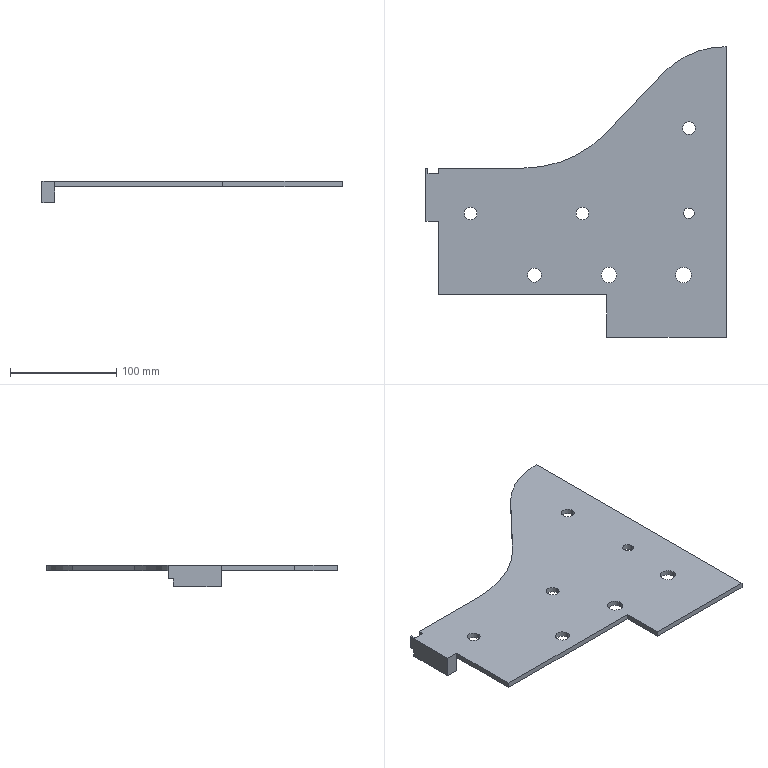Part | SolidWorks | features ICE 3, Cut 2, Extrusion 1 | 1 solid | 34 faces | box 282 x 273 x 20 mm | volume 241277 mm3 | plane 18 | cylinder 16 | commonest cylinder face diameters 12 x6 10 x2 13.206 x2 14.603 x2 14.666 x2 166 x1
STEP:
#1=CARTESIAN_POINT('',(55.96,-170.411,0.));
#2=VERTEX_POINT('',#1);
#3=CARTESIAN_POINT('',(70.625,-170.411,0.));
#4=VERTEX_POINT('',#3);
#5=CARTESIAN_POINT('',(63.293,-170.411,0.));
#6=DIRECTION('',(0.,0.,1.));
#7=DIRECTION('',(1.,0.,0.));
#8=AXIS2_PLACEMENT_3D('',#5,#6,#7);
#9=CIRCLE('',#8,7.333);
#10=EDGE_CURVE('',#2,#4,#9,.T.);
#11=ORIENTED_EDGE('',*,*,#10,.F.);
#12=CARTESIAN_POINT('',(55.96,-170.411,5.));
#13=VERTEX_POINT('',#12);
#14=CARTESIAN_POINT('',(55.96,-170.411,-50.741));
#15=DIRECTION('',(0.,0.,1.));
#16=VECTOR('',#15,1000.);
#17=LINE('',#14,#16);
#18=EDGE_CURVE('',#2,#13,#17,.T.);
#19=ORIENTED_EDGE('',*,*,#18,.T.);
#20=CARTESIAN_POINT('',(70.625,-170.411,5.));
#21=VERTEX_POINT('',#20);
#22=CARTESIAN_POINT('',(63.293,-170.411,5.));
#23=DIRECTION('',(0.,0.,1.));
#24=DIRECTION('',(1.,0.,0.));
#25=AXIS2_PLACEMENT_3D('',#22,#23,#24);
#26=CIRCLE('',#25,7.333);
#27=EDGE_CURVE('',#13,#21,#26,.T.);
#28=ORIENTED_EDGE('',*,*,#27,.T.);
#29=CARTESIAN_POINT('',(70.625,-170.411,-50.741));
#30=DIRECTION('',(0.,0.,1.));
#31=VECTOR('',#30,1000.);
#32=LINE('',#29,#31);
#33=EDGE_CURVE('',#4,#21,#32,.T.);
#34=ORIENTED_EDGE('',*,*,#33,.F.);
#35=EDGE_LOOP('',(#11,#19,#28,#34));
#36=FACE_OUTER_BOUND('',#35,.T.);
#37=CARTESIAN_POINT('',(63.293,-170.411,-50.741));
#38=DIRECTION('',(0.,0.,1.));
#39=DIRECTION('',(1.,0.,0.));
#40=AXIS2_PLACEMENT_3D('',#37,#38,#39);
#41=CYLINDRICAL_SURFACE('',#40,7.333);
#42=ADVANCED_FACE('',(#36),#41,.F.);
#43=CARTESIAN_POINT('',(-14.009,-170.411,0.));
#44=VERTEX_POINT('',#43);
#45=CARTESIAN_POINT('',(0.5938,-170.411,0.));
#46=VERTEX_POINT('',#45);
#47=CARTESIAN_POINT('',(-6.707,-170.411,0.));
#48=DIRECTION('',(0.,0.,1.));
#49=DIRECTION('',(1.,0.,0.));
#50=AXIS2_PLACEMENT_3D('',#47,#48,#49);
#51=CIRCLE('',#50,7.301);
#52=EDGE_CURVE('',#44,#46,#51,.T.);
#53=ORIENTED_EDGE('',*,*,#52,.F.);
#54=CARTESIAN_POINT('',(-14.009,-170.411,5.));
#55=VERTEX_POINT('',#54);
#56=CARTESIAN_POINT('',(-14.009,-170.411,-50.741));
#57=DIRECTION('',(0.,0.,1.));
#58=VECTOR('',#57,1000.);
#59=LINE('',#56,#58);
#60=EDGE_CURVE('',#44,#55,#59,.T.);
#61=ORIENTED_EDGE('',*,*,#60,.T.);
#62=CARTESIAN_POINT('',(0.5938,-170.411,5.));
#63=VERTEX_POINT('',#62);
#64=CARTESIAN_POINT('',(-6.707,-170.411,5.));
#65=DIRECTION('',(0.,0.,1.));
#66=DIRECTION('',(1.,0.,0.));
#67=AXIS2_PLACEMENT_3D('',#64,#65,#66);
#68=CIRCLE('',#67,7.301);
#69=EDGE_CURVE('',#55,#63,#68,.T.);
#70=ORIENTED_EDGE('',*,*,#69,.T.);
#71=CARTESIAN_POINT('',(0.5938,-170.411,-50.741));
#72=DIRECTION('',(0.,0.,1.));
#73=VECTOR('',#72,1000.);
#74=LINE('',#71,#73);
#75=EDGE_CURVE('',#46,#63,#74,.T.);
#76=ORIENTED_EDGE('',*,*,#75,.F.);
#77=EDGE_LOOP('',(#53,#61,#70,#76));
#78=FACE_OUTER_BOUND('',#77,.T.);
#79=CARTESIAN_POINT('',(-6.707,-170.411,-50.741));
#80=DIRECTION('',(0.,0.,1.));
#81=DIRECTION('',(1.,0.,0.));
#82=AXIS2_PLACEMENT_3D('',#79,#80,#81);
#83=CYLINDRICAL_SURFACE('',#82,7.301);
#84=ADVANCED_FACE('',(#78),#83,.F.);
#85=CARTESIAN_POINT('',(-83.311,-170.411,0.));
#86=VERTEX_POINT('',#85);
#87=CARTESIAN_POINT('',(-70.104,-170.411,0.));
#88=VERTEX_POINT('',#87);
#89=CARTESIAN_POINT('',(-76.707,-170.411,0.));
#90=DIRECTION('',(0.,0.,1.));
#91=DIRECTION('',(1.,0.,0.));
#92=AXIS2_PLACEMENT_3D('',#89,#90,#91);
#93=CIRCLE('',#92,6.603);
#94=EDGE_CURVE('',#86,#88,#93,.T.);
#95=ORIENTED_EDGE('',*,*,#94,.F.);
#96=CARTESIAN_POINT('',(-83.311,-170.411,5.));
#97=VERTEX_POINT('',#96);
#98=CARTESIAN_POINT('',(-83.311,-170.411,-50.741));
#99=DIRECTION('',(0.,0.,1.));
#100=VECTOR('',#99,1000.);
#101=LINE('',#98,#100);
#102=EDGE_CURVE('',#86,#97,#101,.T.);
#103=ORIENTED_EDGE('',*,*,#102,.T.);
#104=CARTESIAN_POINT('',(-70.104,-170.411,5.));
#105=VERTEX_POINT('',#104);
#106=CARTESIAN_POINT('',(-76.707,-170.411,5.));
#107=DIRECTION('',(0.,0.,1.));
#108=DIRECTION('',(1.,0.,0.));
#109=AXIS2_PLACEMENT_3D('',#106,#107,#108);
#110=CIRCLE('',#109,6.603);
#111=EDGE_CURVE('',#97,#105,#110,.T.);
#112=ORIENTED_EDGE('',*,*,#111,.T.);
#113=CARTESIAN_POINT('',(-70.104,-170.411,-50.741));
#114=DIRECTION('',(0.,0.,1.));
#115=VECTOR('',#114,1000.);
#116=LINE('',#113,#115);
#117=EDGE_CURVE('',#88,#105,#116,.T.);
#118=ORIENTED_EDGE('',*,*,#117,.F.);
#119=EDGE_LOOP('',(#95,#103,#112,#118));
#120=FACE_OUTER_BOUND('',#119,.T.);
#121=CARTESIAN_POINT('',(-76.707,-170.411,-50.741));
#122=DIRECTION('',(0.,0.,1.));
#123=DIRECTION('',(1.,0.,0.));
#124=AXIS2_PLACEMENT_3D('',#121,#122,#123);
#125=CYLINDRICAL_SURFACE('',#124,6.603);
#126=ADVANCED_FACE('',(#120),#125,.F.);
#127=CARTESIAN_POINT('',(62.293,-32.472,0.));
#128=VERTEX_POINT('',#127);
#129=CARTESIAN_POINT('',(74.293,-32.472,0.));
#130=VERTEX_POINT('',#129);
#131=CARTESIAN_POINT('',(68.293,-32.472,0.));
#132=DIRECTION('',(0.,0.,1.));
#133=DIRECTION('',(1.,0.,0.));
#134=AXIS2_PLACEMENT_3D('',#131,#132,#133);
#135=CIRCLE('',#134,6.);
#136=EDGE_CURVE('',#128,#130,#135,.T.);
#137=ORIENTED_EDGE('',*,*,#136,.F.);
#138=CARTESIAN_POINT('',(62.293,-32.472,5.));
#139=VERTEX_POINT('',#138);
#140=CARTESIAN_POINT('',(62.293,-32.472,-36.971));
#141=DIRECTION('',(0.,0.,1.));
#142=VECTOR('',#141,1000.);
#143=LINE('',#140,#142);
#144=EDGE_CURVE('',#128,#139,#143,.T.);
#145=ORIENTED_EDGE('',*,*,#144,.T.);
#146=CARTESIAN_POINT('',(74.293,-32.472,5.));
#147=VERTEX_POINT('',#146);
#148=CARTESIAN_POINT('',(68.293,-32.472,5.));
#149=DIRECTION('',(0.,0.,1.));
#150=DIRECTION('',(1.,0.,0.));
#151=AXIS2_PLACEMENT_3D('',#148,#149,#150);
#152=CIRCLE('',#151,6.);
#153=EDGE_CURVE('',#139,#147,#152,.T.);
#154=ORIENTED_EDGE('',*,*,#153,.T.);
#155=CARTESIAN_POINT('',(74.293,-32.472,-36.971));
#156=DIRECTION('',(0.,0.,1.));
#157=VECTOR('',#156,1000.);
#158=LINE('',#155,#157);
#159=EDGE_CURVE('',#130,#147,#158,.T.);
#160=ORIENTED_EDGE('',*,*,#159,.F.);
#161=EDGE_LOOP('',(#137,#145,#154,#160));
#162=FACE_OUTER_BOUND('',#161,.T.);
#163=CARTESIAN_POINT('',(68.293,-32.472,-36.971));
#164=DIRECTION('',(0.,0.,1.));
#165=DIRECTION('',(1.,0.,0.));
#166=AXIS2_PLACEMENT_3D('',#163,#164,#165);
#167=CYLINDRICAL_SURFACE('',#166,6.);
#168=ADVANCED_FACE('',(#162),#167,.F.);
#169=CARTESIAN_POINT('',(-142.707,-112.472,0.));
#170=VERTEX_POINT('',#169);
#171=CARTESIAN_POINT('',(-130.707,-112.472,0.));
#172=VERTEX_POINT('',#171);
#173=CARTESIAN_POINT('',(-136.707,-112.472,0.));
#174=DIRECTION('',(0.,0.,1.));
#175=DIRECTION('',(1.,0.,0.));
#176=AXIS2_PLACEMENT_3D('',#173,#174,#175);
#177=CIRCLE('',#176,6.);
#178=EDGE_CURVE('',#170,#172,#177,.T.);
#179=ORIENTED_EDGE('',*,*,#178,.F.);
#180=CARTESIAN_POINT('',(-142.707,-112.472,5.));
#181=VERTEX_POINT('',#180);
#182=CARTESIAN_POINT('',(-142.707,-112.472,-36.971));
#183=DIRECTION('',(0.,0.,1.));
#184=VECTOR('',#183,1000.);
#185=LINE('',#182,#184);
#186=EDGE_CURVE('',#170,#181,#185,.T.);
#187=ORIENTED_EDGE('',*,*,#186,.T.);
#188=CARTESIAN_POINT('',(-130.707,-112.472,5.));
#189=VERTEX_POINT('',#188);
#190=CARTESIAN_POINT('',(-136.707,-112.472,5.));
#191=DIRECTION('',(0.,0.,1.));
#192=DIRECTION('',(1.,0.,0.));
#193=AXIS2_PLACEMENT_3D('',#190,#191,#192);
#194=CIRCLE('',#193,6.);
#195=EDGE_CURVE('',#181,#189,#194,.T.);
#196=ORIENTED_EDGE('',*,*,#195,.T.);
#197=CARTESIAN_POINT('',(-130.707,-112.472,-36.971));
#198=DIRECTION('',(0.,0.,1.));
#199=VECTOR('',#198,1000.);
#200=LINE('',#197,#199);
#201=EDGE_CURVE('',#172,#189,#200,.T.);
#202=ORIENTED_EDGE('',*,*,#201,.F.);
#203=EDGE_LOOP('',(#179,#187,#196,#202));
#204=FACE_OUTER_BOUND('',#203,.T.);
#205=CARTESIAN_POINT('',(-136.707,-112.472,-36.971));
#206=DIRECTION('',(0.,0.,1.));
#207=DIRECTION('',(1.,0.,0.));
#208=AXIS2_PLACEMENT_3D('',#205,#206,#207);
#209=CYLINDRICAL_SURFACE('',#208,6.);
#210=ADVANCED_FACE('',(#204),#209,.F.);
#211=CARTESIAN_POINT('',(-37.707,-112.472,0.));
#212=VERTEX_POINT('',#211);
#213=CARTESIAN_POINT('',(-25.707,-112.472,0.));
#214=VERTEX_POINT('',#213);
#215=CARTESIAN_POINT('',(-31.707,-112.472,0.));
#216=DIRECTION('',(0.,0.,1.));
#217=DIRECTION('',(1.,0.,0.));
#218=AXIS2_PLACEMENT_3D('',#215,#216,#217);
#219=CIRCLE('',#218,6.);
#220=EDGE_CURVE('',#212,#214,#219,.T.);
#221=ORIENTED_EDGE('',*,*,#220,.F.);
#222=CARTESIAN_POINT('',(-37.707,-112.472,5.));
#223=VERTEX_POINT('',#222);
#224=CARTESIAN_POINT('',(-37.707,-112.472,-36.971));
#225=DIRECTION('',(0.,0.,1.));
#226=VECTOR('',#225,1000.);
#227=LINE('',#224,#226);
#228=EDGE_CURVE('',#212,#223,#227,.T.);
#229=ORIENTED_EDGE('',*,*,#228,.T.);
#230=CARTESIAN_POINT('',(-25.707,-112.472,5.));
#231=VERTEX_POINT('',#230);
#232=CARTESIAN_POINT('',(-31.707,-112.472,5.));
#233=DIRECTION('',(0.,0.,1.));
#234=DIRECTION('',(1.,0.,0.));
#235=AXIS2_PLACEMENT_3D('',#232,#233,#234);
#236=CIRCLE('',#235,6.);
#237=EDGE_CURVE('',#223,#231,#236,.T.);
#238=ORIENTED_EDGE('',*,*,#237,.T.);
#239=CARTESIAN_POINT('',(-25.707,-112.472,-36.971));
#240=DIRECTION('',(0.,0.,1.));
#241=VECTOR('',#240,1000.);
#242=LINE('',#239,#241);
#243=EDGE_CURVE('',#214,#231,#242,.T.);
#244=ORIENTED_EDGE('',*,*,#243,.F.);
#245=EDGE_LOOP('',(#221,#229,#238,#244));
#246=FACE_OUTER_BOUND('',#245,.T.);
#247=CARTESIAN_POINT('',(-31.707,-112.472,-36.971));
#248=DIRECTION('',(0.,0.,1.));
#249=DIRECTION('',(1.,0.,0.));
#250=AXIS2_PLACEMENT_3D('',#247,#248,#249);
#251=CYLINDRICAL_SURFACE('',#250,6.);
#252=ADVANCED_FACE('',(#246),#251,.F.);
#253=CARTESIAN_POINT('',(63.293,-112.472,0.));
#254=VERTEX_POINT('',#253);
#255=CARTESIAN_POINT('',(73.293,-112.472,0.));
#256=VERTEX_POINT('',#255);
#257=CARTESIAN_POINT('',(68.293,-112.472,0.));
#258=DIRECTION('',(0.,0.,1.));
#259=DIRECTION('',(1.,0.,0.));
#260=AXIS2_PLACEMENT_3D('',#257,#258,#259);
#261=CIRCLE('',#260,5.);
#262=EDGE_CURVE('',#254,#256,#261,.T.);
#263=ORIENTED_EDGE('',*,*,#262,.F.);
#264=CARTESIAN_POINT('',(63.293,-112.472,5.));
#265=VERTEX_POINT('',#264);
#266=CARTESIAN_POINT('',(63.293,-112.472,-36.971));
#267=DIRECTION('',(0.,0.,1.));
#268=VECTOR('',#267,1000.);
#269=LINE('',#266,#268);
#270=EDGE_CURVE('',#254,#265,#269,.T.);
#271=ORIENTED_EDGE('',*,*,#270,.T.);
#272=CARTESIAN_POINT('',(73.293,-112.472,5.));
#273=VERTEX_POINT('',#272);
#274=CARTESIAN_POINT('',(68.293,-112.472,5.));
#275=DIRECTION('',(0.,0.,1.));
#276=DIRECTION('',(1.,0.,0.));
#277=AXIS2_PLACEMENT_3D('',#274,#275,#276);
#278=CIRCLE('',#277,5.);
#279=EDGE_CURVE('',#265,#273,#278,.T.);
#280=ORIENTED_EDGE('',*,*,#279,.T.);
#281=CARTESIAN_POINT('',(73.293,-112.472,-36.971));
#282=DIRECTION('',(0.,0.,1.));
#283=VECTOR('',#282,1000.);
#284=LINE('',#281,#283);
#285=EDGE_CURVE('',#256,#273,#284,.T.);
#286=ORIENTED_EDGE('',*,*,#285,.F.);
#287=EDGE_LOOP('',(#263,#271,#280,#286));
#288=FACE_OUTER_BOUND('',#287,.T.);
#289=CARTESIAN_POINT('',(68.293,-112.472,-36.971));
#290=DIRECTION('',(0.,0.,1.));
#291=DIRECTION('',(1.,0.,0.));
#292=AXIS2_PLACEMENT_3D('',#289,#290,#291);
#293=CYLINDRICAL_SURFACE('',#292,5.);
#294=ADVANCED_FACE('',(#288),#293,.F.);
#295=CARTESIAN_POINT('',(-8.707,-188.911,5.));
#296=VERTEX_POINT('',#295);
#297=CARTESIAN_POINT('',(-8.707,-188.911,0.));
#298=VERTEX_POINT('',#297);
#299=CARTESIAN_POINT('',(-8.707,-188.911,5.));
#300=DIRECTION('',(0.,0.,-1.));
#301=VECTOR('',#300,1000.);
#302=LINE('',#299,#301);
#303=EDGE_CURVE('',#296,#298,#302,.T.);
#304=ORIENTED_EDGE('',*,*,#303,.F.);
#305=CARTESIAN_POINT('',(-166.707,-188.911,5.));
#306=VERTEX_POINT('',#305);
#307=CARTESIAN_POINT('',(-166.707,-188.911,5.));
#308=DIRECTION('',(1.,0.,0.));
#309=VECTOR('',#308,1000.);
#310=LINE('',#307,#309);
#311=EDGE_CURVE('',#306,#296,#310,.T.);
#312=ORIENTED_EDGE('',*,*,#311,.F.);
#313=CARTESIAN_POINT('',(-166.707,-188.911,0.));
#314=VERTEX_POINT('',#313);
#315=CARTESIAN_POINT('',(-166.707,-188.911,5.));
#316=DIRECTION('',(0.,0.,-1.));
#317=VECTOR('',#316,1000.);
#318=LINE('',#315,#317);
#319=EDGE_CURVE('',#306,#314,#318,.T.);
#320=ORIENTED_EDGE('',*,*,#319,.T.);
#321=CARTESIAN_POINT('',(-86.707,-188.911,0.));
#322=DIRECTION('',(1.,0.,0.));
#323=VECTOR('',#322,1000.);
#324=LINE('',#321,#323);
#325=EDGE_CURVE('',#314,#298,#324,.T.);
#326=ORIENTED_EDGE('',*,*,#325,.T.);
#327=EDGE_LOOP('',(#304,#312,#320,#326));
#328=FACE_OUTER_BOUND('',#327,.T.);
#329=CARTESIAN_POINT('',(-86.707,-188.911,5.));
#330=DIRECTION('',(0.,1.,0.));
#331=DIRECTION('',(0.,0.,1.));
#332=AXIS2_PLACEMENT_3D('',#329,#330,#331);
#333=PLANE('',#332);
#334=ADVANCED_FACE('',(#328),#333,.F.);
#335=CARTESIAN_POINT('',(-166.707,-69.911,5.));
#336=VERTEX_POINT('',#335);
#337=CARTESIAN_POINT('',(-166.707,-69.911,0.));
#338=VERTEX_POINT('',#337);
#339=CARTESIAN_POINT('',(-166.707,-69.911,0.));
#340=DIRECTION('',(0.,0.,-1.));
#341=VECTOR('',#340,1000.);
#342=LINE('',#339,#341);
#343=EDGE_CURVE('',#336,#338,#342,.T.);
#344=ORIENTED_EDGE('',*,*,#343,.F.);
#345=CARTESIAN_POINT('',(-86.707,-69.911,5.));
#346=VERTEX_POINT('',#345);
#347=CARTESIAN_POINT('',(-166.707,-69.911,5.));
#348=DIRECTION('',(1.,0.,0.));
#349=VECTOR('',#348,1000.);
#350=LINE('',#347,#349);
#351=EDGE_CURVE('',#336,#346,#350,.T.);
#352=ORIENTED_EDGE('',*,*,#351,.T.);
#353=CARTESIAN_POINT('',(-86.707,-69.911,0.));
#354=VERTEX_POINT('',#353);
#355=CARTESIAN_POINT('',(-86.707,-69.911,5.));
#356=DIRECTION('',(0.,0.,-1.));
#357=VECTOR('',#356,1000.);
#358=LINE('',#355,#357);
#359=EDGE_CURVE('',#346,#354,#358,.T.);
#360=ORIENTED_EDGE('',*,*,#359,.T.);
#361=CARTESIAN_POINT('',(-166.707,-69.911,0.));
#362=DIRECTION('',(1.,0.,0.));
#363=VECTOR('',#362,1000.);
#364=LINE('',#361,#363);
#365=EDGE_CURVE('',#338,#354,#364,.T.);
#366=ORIENTED_EDGE('',*,*,#365,.F.);
#367=EDGE_LOOP('',(#344,#352,#360,#366));
#368=FACE_OUTER_BOUND('',#367,.T.);
#369=CARTESIAN_POINT('',(-166.707,-69.911,5.));
#370=DIRECTION('',(0.,1.,0.));
#371=DIRECTION('',(0.,0.,1.));
#372=AXIS2_PLACEMENT_3D('',#369,#370,#371);
#373=PLANE('',#372);
#374=ADVANCED_FACE('',(#368),#373,.T.);
#375=CARTESIAN_POINT('',(-166.707,-119.911,5.));
#376=VERTEX_POINT('',#375);
#377=CARTESIAN_POINT('',(-166.707,-69.911,5.));
#378=DIRECTION('',(0.,-1.,0.));
#379=VECTOR('',#378,1000.);
#380=LINE('',#377,#379);
#381=EDGE_CURVE('',#376,#306,#380,.T.);
#382=ORIENTED_EDGE('',*,*,#381,.F.);
#383=CARTESIAN_POINT('',(-166.707,-119.911,0.));
#384=VERTEX_POINT('',#383);
#385=CARTESIAN_POINT('',(-166.707,-119.911,5.));
#386=DIRECTION('',(0.,0.,-1.));
#387=VECTOR('',#386,1000.);
#388=LINE('',#385,#387);
#389=EDGE_CURVE('',#376,#384,#388,.T.);
#390=ORIENTED_EDGE('',*,*,#389,.T.);
#391=CARTESIAN_POINT('',(-166.707,-69.911,0.));
#392=DIRECTION('',(0.,-1.,0.));
#393=VECTOR('',#392,1000.);
#394=LINE('',#391,#393);
#395=EDGE_CURVE('',#384,#314,#394,.T.);
#396=ORIENTED_EDGE('',*,*,#395,.T.);
#397=ORIENTED_EDGE('',*,*,#319,.F.);
#398=EDGE_LOOP('',(#382,#390,#396,#397));
#399=FACE_OUTER_BOUND('',#398,.T.);
#400=CARTESIAN_POINT('',(-166.707,-69.911,5.));
#401=DIRECTION('',(1.,0.,0.));
#402=DIRECTION('',(0.,0.,-1.));
#403=AXIS2_PLACEMENT_3D('',#400,#401,#402);
#404=PLANE('',#403);
#405=ADVANCED_FACE('',(#399),#404,.F.);
#406=CARTESIAN_POINT('',(103.293,44.089,0.));
#407=VERTEX_POINT('',#406);
#408=CARTESIAN_POINT('',(103.293,-228.911,0.));
#409=VERTEX_POINT('',#408);
#410=CARTESIAN_POINT('',(103.293,44.089,0.));
#411=DIRECTION('',(0.,-1.,0.));
#412=VECTOR('',#411,1000.);
#413=LINE('',#410,#412);
#414=EDGE_CURVE('',#407,#409,#413,.T.);
#415=ORIENTED_EDGE('',*,*,#414,.F.);
#416=CARTESIAN_POINT('',(103.293,44.089,5.));
#417=VERTEX_POINT('',#416);
#418=CARTESIAN_POINT('',(103.293,44.089,5.));
#419=DIRECTION('',(0.,0.,-1.));
#420=VECTOR('',#419,1000.);
#421=LINE('',#418,#420);
#422=EDGE_CURVE('',#417,#407,#421,.T.);
#423=ORIENTED_EDGE('',*,*,#422,.F.);
#424=CARTESIAN_POINT('',(103.293,-228.911,5.));
#425=VERTEX_POINT('',#424);
#426=CARTESIAN_POINT('',(103.293,44.089,5.));
#427=DIRECTION('',(0.,-1.,0.));
#428=VECTOR('',#427,1000.);
#429=LINE('',#426,#428);
#430=EDGE_CURVE('',#417,#425,#429,.T.);
#431=ORIENTED_EDGE('',*,*,#430,.T.);
#432=CARTESIAN_POINT('',(103.293,-228.911,5.));
#433=DIRECTION('',(0.,0.,1.));
#434=VECTOR('',#433,1000.);
#435=LINE('',#432,#434);
#436=EDGE_CURVE('',#409,#425,#435,.T.);
#437=ORIENTED_EDGE('',*,*,#436,.F.);
#438=EDGE_LOOP('',(#415,#423,#431,#437));
#439=FACE_OUTER_BOUND('',#438,.T.);
#440=CARTESIAN_POINT('',(103.293,44.089,5.));
#441=DIRECTION('',(1.,0.,0.));
#442=DIRECTION('',(0.,0.,-1.));
#443=AXIS2_PLACEMENT_3D('',#440,#441,#442);
#444=PLANE('',#443);
#445=ADVANCED_FACE('',(#439),#444,.T.);
#446=CARTESIAN_POINT('',(44.7,19.876,0.));
#447=VERTEX_POINT('',#446);
#448=CARTESIAN_POINT('',(103.293,-38.911,0.));
#449=DIRECTION('',(0.,0.,1.));
#450=DIRECTION('',(1.,0.,0.));
#451=AXIS2_PLACEMENT_3D('',#448,#449,#450);
#452=CIRCLE('',#451,83.);
#453=EDGE_CURVE('',#407,#447,#452,.T.);
#454=ORIENTED_EDGE('',*,*,#453,.T.);
#455=CARTESIAN_POINT('',(44.7,19.876,5.));
#456=VERTEX_POINT('',#455);
#457=CARTESIAN_POINT('',(44.7,19.876,5.));
#458=DIRECTION('',(0.,0.,-1.));
#459=VECTOR('',#458,1000.);
#460=LINE('',#457,#459);
#461=EDGE_CURVE('',#456,#447,#460,.T.);
#462=ORIENTED_EDGE('',*,*,#461,.F.);
#463=CARTESIAN_POINT('',(103.293,-38.911,5.));
#464=DIRECTION('',(0.,0.,1.));
#465=DIRECTION('',(1.,0.,0.));
#466=AXIS2_PLACEMENT_3D('',#463,#464,#465);
#467=CIRCLE('',#466,83.);
#468=EDGE_CURVE('',#417,#456,#467,.T.);
#469=ORIENTED_EDGE('',*,*,#468,.F.);
#470=ORIENTED_EDGE('',*,*,#422,.T.);
#471=EDGE_LOOP('',(#454,#462,#469,#470));
#472=FACE_OUTER_BOUND('',#471,.T.);
#473=CARTESIAN_POINT('',(103.293,-38.911,5.));
#474=DIRECTION('',(0.,0.,-1.));
#475=DIRECTION('',(-1.,0.,0.));
#476=AXIS2_PLACEMENT_3D('',#473,#474,#475);
#477=CYLINDRICAL_SURFACE('',#476,83.);
#478=ADVANCED_FACE('',(#472),#477,.T.);
#479=CARTESIAN_POINT('',(-10.944,-38.467,0.));
#480=VERTEX_POINT('',#479);
#481=CARTESIAN_POINT('',(-10.944,-38.467,0.));
#482=CARTESIAN_POINT('',(16.878,-9.296,0.));
#483=CARTESIAN_POINT('',(44.7,19.876,0.));
#484=B_SPLINE_CURVE_WITH_KNOTS('',2,(#481,#482,#483),.UNSPECIFIED.,.F.,.F.,(3,3),(-0.00171,0.9982),.UNSPECIFIED.);
#485=EDGE_CURVE('',#480,#447,#484,.T.);
#486=ORIENTED_EDGE('',*,*,#485,.F.);
#487=CARTESIAN_POINT('',(-10.944,-38.467,5.));
#488=VERTEX_POINT('',#487);
#489=CARTESIAN_POINT('',(-10.944,-38.467,5.));
#490=DIRECTION('',(0.,0.,-1.));
#491=VECTOR('',#490,1000.);
#492=LINE('',#489,#491);
#493=EDGE_CURVE('',#488,#480,#492,.T.);
#494=ORIENTED_EDGE('',*,*,#493,.F.);
#495=CARTESIAN_POINT('',(-10.944,-38.467,5.));
#496=CARTESIAN_POINT('',(16.878,-9.296,5.));
#497=CARTESIAN_POINT('',(44.7,19.876,5.));
#498=B_SPLINE_CURVE_WITH_KNOTS('',2,(#495,#496,#497),.UNSPECIFIED.,.F.,.F.,(3,3),(-0.00171,0.9982),.UNSPECIFIED.);
#499=EDGE_CURVE('',#488,#456,#498,.T.);
#500=ORIENTED_EDGE('',*,*,#499,.T.);
#501=ORIENTED_EDGE('',*,*,#461,.T.);
#502=EDGE_LOOP('',(#486,#494,#500,#501));
#503=FACE_OUTER_BOUND('',#502,.T.);
#504=CARTESIAN_POINT('',(-10.944,-38.467,5.));
#505=DIRECTION('',(-0.7237,0.6902,0.));
#506=DIRECTION('',(-0.6902,-0.7237,0.));
#507=AXIS2_PLACEMENT_3D('',#504,#505,#506);
#508=PLANE('',#507);
#509=ADVANCED_FACE('',(#503),#508,.T.);
#510=CARTESIAN_POINT('',(-86.707,37.089,0.));
#511=DIRECTION('',(0.,0.,1.));
#512=DIRECTION('',(1.,0.,0.));
#513=AXIS2_PLACEMENT_3D('',#510,#511,#512);
#514=CIRCLE('',#513,107.);
#515=EDGE_CURVE('',#354,#480,#514,.T.);
#516=ORIENTED_EDGE('',*,*,#515,.F.);
#517=ORIENTED_EDGE('',*,*,#359,.F.);
#518=CARTESIAN_POINT('',(-86.707,37.089,5.));
#519=DIRECTION('',(0.,0.,1.));
#520=DIRECTION('',(1.,0.,0.));
#521=AXIS2_PLACEMENT_3D('',#518,#519,#520);
#522=CIRCLE('',#521,107.);
#523=EDGE_CURVE('',#346,#488,#522,.T.);
#524=ORIENTED_EDGE('',*,*,#523,.T.);
#525=ORIENTED_EDGE('',*,*,#493,.T.);
#526=EDGE_LOOP('',(#516,#517,#524,#525));
#527=FACE_OUTER_BOUND('',#526,.T.);
#528=CARTESIAN_POINT('',(-86.707,37.089,5.));
#529=DIRECTION('',(0.,0.,-1.));
#530=DIRECTION('',(-1.,0.,0.));
#531=AXIS2_PLACEMENT_3D('',#528,#529,#530);
#532=CYLINDRICAL_SURFACE('',#531,107.);
#533=ADVANCED_FACE('',(#527),#532,.F.);
#534=CARTESIAN_POINT('',(-176.72,-69.911,-7.5));
#535=VERTEX_POINT('',#534);
#536=CARTESIAN_POINT('',(-176.72,-69.911,5.));
#537=VERTEX_POINT('',#536);
#538=CARTESIAN_POINT('',(-176.72,-69.911,5.));
#539=DIRECTION('',(0.,0.,1.));
#540=VECTOR('',#539,1000.);
#541=LINE('',#538,#540);
#542=EDGE_CURVE('',#535,#537,#541,.T.);
#543=ORIENTED_EDGE('',*,*,#542,.F.);
#544=CARTESIAN_POINT('',(-178.707,-69.911,-7.5));
#545=VERTEX_POINT('',#544);
#546=CARTESIAN_POINT('',(-176.72,-69.911,-7.5));
#547=DIRECTION('',(1.,0.,0.));
#548=VECTOR('',#547,1000.);
#549=LINE('',#546,#548);
#550=EDGE_CURVE('',#545,#535,#549,.T.);
#551=ORIENTED_EDGE('',*,*,#550,.F.);
#552=CARTESIAN_POINT('',(-178.707,-69.911,5.));
#553=VERTEX_POINT('',#552);
#554=CARTESIAN_POINT('',(-178.707,-69.911,5.));
#555=DIRECTION('',(0.,0.,1.));
#556=VECTOR('',#555,1000.);
#557=LINE('',#554,#556);
#558=EDGE_CURVE('',#545,#553,#557,.T.);
#559=ORIENTED_EDGE('',*,*,#558,.T.);
#560=CARTESIAN_POINT('',(-166.707,-69.911,5.));
#561=DIRECTION('',(1.,0.,0.));
#562=VECTOR('',#561,1000.);
#563=LINE('',#560,#562);
#564=EDGE_CURVE('',#553,#537,#563,.T.);
#565=ORIENTED_EDGE('',*,*,#564,.T.);
#566=EDGE_LOOP('',(#543,#551,#559,#565));
#567=FACE_OUTER_BOUND('',#566,.T.);
#568=CARTESIAN_POINT('',(-166.707,-69.911,5.));
#569=DIRECTION('',(0.,1.,0.));
#570=DIRECTION('',(0.,0.,1.));
#571=AXIS2_PLACEMENT_3D('',#568,#569,#570);
#572=PLANE('',#571);
#573=ADVANCED_FACE('',(#567),#572,.T.);
#574=CARTESIAN_POINT('',(63.293,-170.411,5.));
#575=DIRECTION('',(0.,0.,1.));
#576=DIRECTION('',(1.,0.,0.));
#577=AXIS2_PLACEMENT_3D('',#574,#575,#576);
#578=CIRCLE('',#577,7.333);
#579=EDGE_CURVE('',#21,#13,#578,.T.);
#580=ORIENTED_EDGE('',*,*,#579,.F.);
#581=ORIENTED_EDGE('',*,*,#27,.F.);
#582=EDGE_LOOP('',(#580,#581));
#583=FACE_BOUND('',#582,.T.);
#584=CARTESIAN_POINT('',(-6.707,-170.411,5.));
#585=DIRECTION('',(0.,0.,1.));
#586=DIRECTION('',(1.,0.,0.));
#587=AXIS2_PLACEMENT_3D('',#584,#585,#586);
#588=CIRCLE('',#587,7.301);
#589=EDGE_CURVE('',#63,#55,#588,.T.);
#590=ORIENTED_EDGE('',*,*,#589,.F.);
#591=ORIENTED_EDGE('',*,*,#69,.F.);
#592=EDGE_LOOP('',(#590,#591));
#593=FACE_BOUND('',#592,.T.);
#594=CARTESIAN_POINT('',(-76.707,-170.411,5.));
#595=DIRECTION('',(0.,0.,1.));
#596=DIRECTION('',(1.,0.,0.));
#597=AXIS2_PLACEMENT_3D('',#594,#595,#596);
#598=CIRCLE('',#597,6.603);
#599=EDGE_CURVE('',#105,#97,#598,.T.);
#600=ORIENTED_EDGE('',*,*,#599,.F.);
#601=ORIENTED_EDGE('',*,*,#111,.F.);
#602=EDGE_LOOP('',(#600,#601));
#603=FACE_BOUND('',#602,.T.);
#604=CARTESIAN_POINT('',(68.293,-32.472,5.));
#605=DIRECTION('',(0.,0.,1.));
#606=DIRECTION('',(1.,0.,0.));
#607=AXIS2_PLACEMENT_3D('',#604,#605,#606);
#608=CIRCLE('',#607,6.);
#609=EDGE_CURVE('',#147,#139,#608,.T.);
#610=ORIENTED_EDGE('',*,*,#609,.F.);
#611=ORIENTED_EDGE('',*,*,#153,.F.);
#612=EDGE_LOOP('',(#610,#611));
#613=FACE_BOUND('',#612,.T.);
#614=CARTESIAN_POINT('',(-136.707,-112.472,5.));
#615=DIRECTION('',(0.,0.,1.));
#616=DIRECTION('',(1.,0.,0.));
#617=AXIS2_PLACEMENT_3D('',#614,#615,#616);
#618=CIRCLE('',#617,6.);
#619=EDGE_CURVE('',#189,#181,#618,.T.);
#620=ORIENTED_EDGE('',*,*,#619,.F.);
#621=ORIENTED_EDGE('',*,*,#195,.F.);
#622=EDGE_LOOP('',(#620,#621));
#623=FACE_BOUND('',#622,.T.);
#624=CARTESIAN_POINT('',(-31.707,-112.472,5.));
#625=DIRECTION('',(0.,0.,1.));
#626=DIRECTION('',(1.,0.,0.));
#627=AXIS2_PLACEMENT_3D('',#624,#625,#626);
#628=CIRCLE('',#627,6.);
#629=EDGE_CURVE('',#231,#223,#628,.T.);
#630=ORIENTED_EDGE('',*,*,#629,.F.);
#631=ORIENTED_EDGE('',*,*,#237,.F.);
#632=EDGE_LOOP('',(#630,#631));
#633=FACE_BOUND('',#632,.T.);
#634=CARTESIAN_POINT('',(68.293,-112.472,5.));
#635=DIRECTION('',(0.,0.,1.));
#636=DIRECTION('',(1.,0.,0.));
#637=AXIS2_PLACEMENT_3D('',#634,#635,#636);
#638=CIRCLE('',#637,5.);
#639=EDGE_CURVE('',#273,#265,#638,.T.);
#640=ORIENTED_EDGE('',*,*,#639,.F.);
#641=ORIENTED_EDGE('',*,*,#279,.F.);
#642=EDGE_LOOP('',(#640,#641));
#643=FACE_BOUND('',#642,.T.);
#644=CARTESIAN_POINT('',(-166.707,-74.911,5.));
#645=VERTEX_POINT('',#644);
#646=CARTESIAN_POINT('',(-166.707,-74.911,5.));
#647=DIRECTION('',(0.,1.,0.));
#648=VECTOR('',#647,1000.);
#649=LINE('',#646,#648);
#650=EDGE_CURVE('',#645,#336,#649,.T.);
#651=ORIENTED_EDGE('',*,*,#650,.F.);
#652=CARTESIAN_POINT('',(-176.72,-74.911,5.));
#653=VERTEX_POINT('',#652);
#654=CARTESIAN_POINT('',(-166.707,-74.911,5.));
#655=DIRECTION('',(1.,0.,0.));
#656=VECTOR('',#655,1000.);
#657=LINE('',#654,#656);
#658=EDGE_CURVE('',#653,#645,#657,.T.);
#659=ORIENTED_EDGE('',*,*,#658,.F.);
#660=CARTESIAN_POINT('',(-176.72,-74.911,5.));
#661=DIRECTION('',(0.,1.,0.));
#662=VECTOR('',#661,1000.);
#663=LINE('',#660,#662);
#664=EDGE_CURVE('',#653,#537,#663,.T.);
#665=ORIENTED_EDGE('',*,*,#664,.T.);
#666=ORIENTED_EDGE('',*,*,#564,.F.);
#667=CARTESIAN_POINT('',(-178.707,-119.911,5.));
#668=VERTEX_POINT('',#667);
#669=CARTESIAN_POINT('',(-178.707,-119.911,5.));
#670=DIRECTION('',(0.,1.,0.));
#671=VECTOR('',#670,1000.);
#672=LINE('',#669,#671);
#673=EDGE_CURVE('',#668,#553,#672,.T.);
#674=ORIENTED_EDGE('',*,*,#673,.F.);
#675=CARTESIAN_POINT('',(-166.707,-119.911,5.));
#676=DIRECTION('',(1.,0.,0.));
#677=VECTOR('',#676,1000.);
#678=LINE('',#675,#677);
#679=EDGE_CURVE('',#668,#376,#678,.T.);
#680=ORIENTED_EDGE('',*,*,#679,.T.);
#681=ORIENTED_EDGE('',*,*,#381,.T.);
#682=ORIENTED_EDGE('',*,*,#311,.T.);
#683=CARTESIAN_POINT('',(-8.707,-228.911,5.));
#684=VERTEX_POINT('',#683);
#685=CARTESIAN_POINT('',(-8.707,-228.911,5.));
#686=DIRECTION('',(0.,1.,0.));
#687=VECTOR('',#686,1000.);
#688=LINE('',#685,#687);
#689=EDGE_CURVE('',#684,#296,#688,.T.);
#690=ORIENTED_EDGE('',*,*,#689,.F.);
#691=CARTESIAN_POINT('',(103.293,-228.911,5.));
#692=DIRECTION('',(-1.,0.,0.));
#693=VECTOR('',#692,1000.);
#694=LINE('',#691,#693);
#695=EDGE_CURVE('',#425,#684,#694,.T.);
#696=ORIENTED_EDGE('',*,*,#695,.F.);
#697=ORIENTED_EDGE('',*,*,#430,.F.);
#698=ORIENTED_EDGE('',*,*,#468,.T.);
#699=ORIENTED_EDGE('',*,*,#499,.F.);
#700=ORIENTED_EDGE('',*,*,#523,.F.);
#701=ORIENTED_EDGE('',*,*,#351,.F.);
#702=EDGE_LOOP('',(#651,#659,#665,#666,#674,#680,#681,#682,#690,#696,#697,#698,#699,#700,#701));
#703=FACE_OUTER_BOUND('',#702,.T.);
#704=CARTESIAN_POINT('',(103.293,-38.911,5.));
#705=DIRECTION('',(0.,0.,1.));
#706=DIRECTION('',(1.,0.,0.));
#707=AXIS2_PLACEMENT_3D('',#704,#705,#706);
#708=PLANE('',#707);
#709=ADVANCED_FACE('',(#583,#593,#603,#613,#623,#633,#643,#703),#708,.T.);
#710=CARTESIAN_POINT('',(63.293,-170.411,0.));
#711=DIRECTION('',(0.,0.,1.));
#712=DIRECTION('',(1.,0.,0.));
#713=AXIS2_PLACEMENT_3D('',#710,#711,#712);
#714=CIRCLE('',#713,7.333);
#715=EDGE_CURVE('',#4,#2,#714,.T.);
#716=ORIENTED_EDGE('',*,*,#715,.T.);
#717=ORIENTED_EDGE('',*,*,#10,.T.);
#718=EDGE_LOOP('',(#716,#717));
#719=FACE_BOUND('',#718,.T.);
#720=CARTESIAN_POINT('',(-6.707,-170.411,0.));
#721=DIRECTION('',(0.,0.,1.));
#722=DIRECTION('',(1.,0.,0.));
#723=AXIS2_PLACEMENT_3D('',#720,#721,#722);
#724=CIRCLE('',#723,7.301);
#725=EDGE_CURVE('',#46,#44,#724,.T.);
#726=ORIENTED_EDGE('',*,*,#725,.T.);
#727=ORIENTED_EDGE('',*,*,#52,.T.);
#728=EDGE_LOOP('',(#726,#727));
#729=FACE_BOUND('',#728,.T.);
#730=CARTESIAN_POINT('',(-76.707,-170.411,0.));
#731=DIRECTION('',(0.,0.,1.));
#732=DIRECTION('',(1.,0.,0.));
#733=AXIS2_PLACEMENT_3D('',#730,#731,#732);
#734=CIRCLE('',#733,6.603);
#735=EDGE_CURVE('',#88,#86,#734,.T.);
#736=ORIENTED_EDGE('',*,*,#735,.T.);
#737=ORIENTED_EDGE('',*,*,#94,.T.);
#738=EDGE_LOOP('',(#736,#737));
#739=FACE_BOUND('',#738,.T.);
#740=CARTESIAN_POINT('',(68.293,-32.472,0.));
#741=DIRECTION('',(0.,0.,1.));
#742=DIRECTION('',(1.,0.,0.));
#743=AXIS2_PLACEMENT_3D('',#740,#741,#742);
#744=CIRCLE('',#743,6.);
#745=EDGE_CURVE('',#130,#128,#744,.T.);
#746=ORIENTED_EDGE('',*,*,#745,.T.);
#747=ORIENTED_EDGE('',*,*,#136,.T.);
#748=EDGE_LOOP('',(#746,#747));
#749=FACE_BOUND('',#748,.T.);
#750=CARTESIAN_POINT('',(-136.707,-112.472,0.));
#751=DIRECTION('',(0.,0.,1.));
#752=DIRECTION('',(1.,0.,0.));
#753=AXIS2_PLACEMENT_3D('',#750,#751,#752);
#754=CIRCLE('',#753,6.);
#755=EDGE_CURVE('',#172,#170,#754,.T.);
#756=ORIENTED_EDGE('',*,*,#755,.T.);
#757=ORIENTED_EDGE('',*,*,#178,.T.);
#758=EDGE_LOOP('',(#756,#757));
#759=FACE_BOUND('',#758,.T.);
#760=CARTESIAN_POINT('',(-31.707,-112.472,0.));
#761=DIRECTION('',(0.,0.,1.));
#762=DIRECTION('',(1.,0.,0.));
#763=AXIS2_PLACEMENT_3D('',#760,#761,#762);
#764=CIRCLE('',#763,6.);
#765=EDGE_CURVE('',#214,#212,#764,.T.);
#766=ORIENTED_EDGE('',*,*,#765,.T.);
#767=ORIENTED_EDGE('',*,*,#220,.T.);
#768=EDGE_LOOP('',(#766,#767));
#769=FACE_BOUND('',#768,.T.);
#770=CARTESIAN_POINT('',(68.293,-112.472,0.));
#771=DIRECTION('',(0.,0.,1.));
#772=DIRECTION('',(1.,0.,0.));
#773=AXIS2_PLACEMENT_3D('',#770,#771,#772);
#774=CIRCLE('',#773,5.);
#775=EDGE_CURVE('',#256,#254,#774,.T.);
#776=ORIENTED_EDGE('',*,*,#775,.T.);
#777=ORIENTED_EDGE('',*,*,#262,.T.);
#778=EDGE_LOOP('',(#776,#777));
#779=FACE_BOUND('',#778,.T.);
#780=CARTESIAN_POINT('',(-166.707,-74.911,0.));
#781=VERTEX_POINT('',#780);
#782=CARTESIAN_POINT('',(-166.707,-69.911,0.));
#783=DIRECTION('',(0.,-1.,0.));
#784=VECTOR('',#783,1000.);
#785=LINE('',#782,#784);
#786=EDGE_CURVE('',#338,#781,#785,.T.);
#787=ORIENTED_EDGE('',*,*,#786,.F.);
#788=ORIENTED_EDGE('',*,*,#365,.T.);
#789=ORIENTED_EDGE('',*,*,#515,.T.);
#790=ORIENTED_EDGE('',*,*,#485,.T.);
#791=ORIENTED_EDGE('',*,*,#453,.F.);
#792=ORIENTED_EDGE('',*,*,#414,.T.);
#793=CARTESIAN_POINT('',(-8.707,-228.911,0.));
#794=VERTEX_POINT('',#793);
#795=CARTESIAN_POINT('',(103.293,-228.911,0.));
#796=DIRECTION('',(1.,0.,0.));
#797=VECTOR('',#796,1000.);
#798=LINE('',#795,#797);
#799=EDGE_CURVE('',#794,#409,#798,.T.);
#800=ORIENTED_EDGE('',*,*,#799,.F.);
#801=CARTESIAN_POINT('',(-8.707,-228.911,0.));
#802=DIRECTION('',(0.,1.,0.));
#803=VECTOR('',#802,1000.);
#804=LINE('',#801,#803);
#805=EDGE_CURVE('',#794,#298,#804,.T.);
#806=ORIENTED_EDGE('',*,*,#805,.T.);
#807=ORIENTED_EDGE('',*,*,#325,.F.);
#808=ORIENTED_EDGE('',*,*,#395,.F.);
#809=CARTESIAN_POINT('',(-166.707,-69.911,0.));
#810=DIRECTION('',(0.,-1.,0.));
#811=VECTOR('',#810,1000.);
#812=LINE('',#809,#811);
#813=EDGE_CURVE('',#781,#384,#812,.T.);
#814=ORIENTED_EDGE('',*,*,#813,.F.);
#815=EDGE_LOOP('',(#787,#788,#789,#790,#791,#792,#800,#806,#807,#808,#814));
#816=FACE_OUTER_BOUND('',#815,.T.);
#817=CARTESIAN_POINT('',(103.293,-38.911,0.));
#818=DIRECTION('',(0.,0.,1.));
#819=DIRECTION('',(1.,0.,0.));
#820=AXIS2_PLACEMENT_3D('',#817,#818,#819);
#821=PLANE('',#820);
#822=ADVANCED_FACE('',(#719,#729,#739,#749,#759,#769,#779,#816),#821,.F.);
#823=CARTESIAN_POINT('',(-166.707,-74.911,-15.));
#824=VERTEX_POINT('',#823);
#825=CARTESIAN_POINT('',(-166.707,-74.911,-15.));
#826=DIRECTION('',(0.,0.,-1.));
#827=VECTOR('',#826,1000.);
#828=LINE('',#825,#827);
#829=EDGE_CURVE('',#781,#824,#828,.T.);
#830=ORIENTED_EDGE('',*,*,#829,.F.);
#831=ORIENTED_EDGE('',*,*,#813,.T.);
#832=CARTESIAN_POINT('',(-166.707,-119.911,-15.));
#833=VERTEX_POINT('',#832);
#834=CARTESIAN_POINT('',(-166.707,-119.911,5.));
#835=DIRECTION('',(0.,0.,-1.));
#836=VECTOR('',#835,1000.);
#837=LINE('',#834,#836);
#838=EDGE_CURVE('',#384,#833,#837,.T.);
#839=ORIENTED_EDGE('',*,*,#838,.T.);
#840=CARTESIAN_POINT('',(-166.707,-119.911,-15.));
#841=DIRECTION('',(0.,1.,0.));
#842=VECTOR('',#841,1000.);
#843=LINE('',#840,#842);
#844=EDGE_CURVE('',#833,#824,#843,.T.);
#845=ORIENTED_EDGE('',*,*,#844,.T.);
#846=EDGE_LOOP('',(#830,#831,#839,#845));
#847=FACE_OUTER_BOUND('',#846,.T.);
#848=CARTESIAN_POINT('',(-166.707,-119.911,5.));
#849=DIRECTION('',(1.,0.,0.));
#850=DIRECTION('',(0.,0.,-1.));
#851=AXIS2_PLACEMENT_3D('',#848,#849,#850);
#852=PLANE('',#851);
#853=ADVANCED_FACE('',(#847),#852,.T.);
#854=CARTESIAN_POINT('',(-178.707,-74.911,-7.5));
#855=VERTEX_POINT('',#854);
#856=CARTESIAN_POINT('',(-178.707,-74.911,-7.5));
#857=DIRECTION('',(0.,1.,0.));
#858=VECTOR('',#857,1000.);
#859=LINE('',#856,#858);
#860=EDGE_CURVE('',#855,#545,#859,.T.);
#861=ORIENTED_EDGE('',*,*,#860,.F.);
#862=CARTESIAN_POINT('',(-178.707,-74.911,-15.));
#863=VERTEX_POINT('',#862);
#864=CARTESIAN_POINT('',(-178.707,-74.911,-7.5));
#865=DIRECTION('',(0.,0.,1.));
#866=VECTOR('',#865,1000.);
#867=LINE('',#864,#866);
#868=EDGE_CURVE('',#863,#855,#867,.T.);
#869=ORIENTED_EDGE('',*,*,#868,.F.);
#870=CARTESIAN_POINT('',(-178.707,-119.911,-15.));
#871=VERTEX_POINT('',#870);
#872=CARTESIAN_POINT('',(-178.707,-119.911,-15.));
#873=DIRECTION('',(0.,1.,0.));
#874=VECTOR('',#873,1000.);
#875=LINE('',#872,#874);
#876=EDGE_CURVE('',#871,#863,#875,.T.);
#877=ORIENTED_EDGE('',*,*,#876,.F.);
#878=CARTESIAN_POINT('',(-178.707,-119.911,5.));
#879=DIRECTION('',(0.,0.,1.));
#880=VECTOR('',#879,1000.);
#881=LINE('',#878,#880);
#882=EDGE_CURVE('',#871,#668,#881,.T.);
#883=ORIENTED_EDGE('',*,*,#882,.T.);
#884=ORIENTED_EDGE('',*,*,#673,.T.);
#885=ORIENTED_EDGE('',*,*,#558,.F.);
#886=EDGE_LOOP('',(#861,#869,#877,#883,#884,#885));
#887=FACE_OUTER_BOUND('',#886,.T.);
#888=CARTESIAN_POINT('',(-178.707,-119.911,5.));
#889=DIRECTION('',(-1.,0.,0.));
#890=DIRECTION('',(0.,0.,1.));
#891=AXIS2_PLACEMENT_3D('',#888,#889,#890);
#892=PLANE('',#891);
#893=ADVANCED_FACE('',(#887),#892,.T.);
#894=CARTESIAN_POINT('',(-178.707,-74.911,-15.));
#895=DIRECTION('',(-1.,0.,0.));
#896=VECTOR('',#895,1000.);
#897=LINE('',#894,#896);
#898=EDGE_CURVE('',#824,#863,#897,.T.);
#899=ORIENTED_EDGE('',*,*,#898,.F.);
#900=ORIENTED_EDGE('',*,*,#844,.F.);
#901=CARTESIAN_POINT('',(-166.707,-119.911,-15.));
#902=DIRECTION('',(-1.,0.,0.));
#903=VECTOR('',#902,1000.);
#904=LINE('',#901,#903);
#905=EDGE_CURVE('',#833,#871,#904,.T.);
#906=ORIENTED_EDGE('',*,*,#905,.T.);
#907=ORIENTED_EDGE('',*,*,#876,.T.);
#908=EDGE_LOOP('',(#899,#900,#906,#907));
#909=FACE_OUTER_BOUND('',#908,.T.);
#910=CARTESIAN_POINT('',(-166.707,-119.911,-15.));
#911=DIRECTION('',(0.,0.,-1.));
#912=DIRECTION('',(-1.,0.,0.));
#913=AXIS2_PLACEMENT_3D('',#910,#911,#912);
#914=PLANE('',#913);
#915=ADVANCED_FACE('',(#909),#914,.T.);
#916=ORIENTED_EDGE('',*,*,#389,.F.);
#917=ORIENTED_EDGE('',*,*,#679,.F.);
#918=ORIENTED_EDGE('',*,*,#882,.F.);
#919=ORIENTED_EDGE('',*,*,#905,.F.);
#920=ORIENTED_EDGE('',*,*,#838,.F.);
#921=EDGE_LOOP('',(#916,#917,#918,#919,#920));
#922=FACE_OUTER_BOUND('',#921,.T.);
#923=CARTESIAN_POINT('',(0.,-119.911,0.));
#924=DIRECTION('',(0.,1.,0.));
#925=DIRECTION('',(0.,0.,1.));
#926=AXIS2_PLACEMENT_3D('',#923,#924,#925);
#927=PLANE('',#926);
#928=ADVANCED_FACE('',(#922),#927,.F.);
#929=CARTESIAN_POINT('',(-166.707,-74.911,-15.));
#930=DIRECTION('',(0.,0.,-1.));
#931=VECTOR('',#930,1000.);
#932=LINE('',#929,#931);
#933=EDGE_CURVE('',#645,#781,#932,.T.);
#934=ORIENTED_EDGE('',*,*,#933,.F.);
#935=ORIENTED_EDGE('',*,*,#650,.T.);
#936=ORIENTED_EDGE('',*,*,#343,.T.);
#937=ORIENTED_EDGE('',*,*,#786,.T.);
#938=EDGE_LOOP('',(#934,#935,#936,#937));
#939=FACE_OUTER_BOUND('',#938,.T.);
#940=CARTESIAN_POINT('',(-166.707,-74.911,0.));
#941=DIRECTION('',(1.,0.,0.));
#942=DIRECTION('',(0.,0.,-1.));
#943=AXIS2_PLACEMENT_3D('',#940,#941,#942);
#944=PLANE('',#943);
#945=ADVANCED_FACE('',(#939),#944,.F.);
#946=ORIENTED_EDGE('',*,*,#542,.T.);
#947=ORIENTED_EDGE('',*,*,#664,.F.);
#948=CARTESIAN_POINT('',(-176.72,-74.911,-7.5));
#949=VERTEX_POINT('',#948);
#950=CARTESIAN_POINT('',(-176.72,-74.911,5.));
#951=DIRECTION('',(0.,0.,1.));
#952=VECTOR('',#951,1000.);
#953=LINE('',#950,#952);
#954=EDGE_CURVE('',#949,#653,#953,.T.);
#955=ORIENTED_EDGE('',*,*,#954,.F.);
#956=CARTESIAN_POINT('',(-176.72,-74.911,-7.5));
#957=DIRECTION('',(0.,1.,0.));
#958=VECTOR('',#957,1000.);
#959=LINE('',#956,#958);
#960=EDGE_CURVE('',#949,#535,#959,.T.);
#961=ORIENTED_EDGE('',*,*,#960,.T.);
#962=EDGE_LOOP('',(#946,#947,#955,#961));
#963=FACE_OUTER_BOUND('',#962,.T.);
#964=CARTESIAN_POINT('',(-176.72,-74.911,5.));
#965=DIRECTION('',(-1.,0.,0.));
#966=DIRECTION('',(0.,0.,1.));
#967=AXIS2_PLACEMENT_3D('',#964,#965,#966);
#968=PLANE('',#967);
#969=ADVANCED_FACE('',(#963),#968,.F.);
#970=ORIENTED_EDGE('',*,*,#550,.T.);
#971=ORIENTED_EDGE('',*,*,#960,.F.);
#972=CARTESIAN_POINT('',(-176.72,-74.911,-7.5));
#973=DIRECTION('',(1.,0.,0.));
#974=VECTOR('',#973,1000.);
#975=LINE('',#972,#974);
#976=EDGE_CURVE('',#855,#949,#975,.T.);
#977=ORIENTED_EDGE('',*,*,#976,.F.);
#978=ORIENTED_EDGE('',*,*,#860,.T.);
#979=EDGE_LOOP('',(#970,#971,#977,#978));
#980=FACE_OUTER_BOUND('',#979,.T.);
#981=CARTESIAN_POINT('',(-176.72,-74.911,-7.5));
#982=DIRECTION('',(0.,0.,1.));
#983=DIRECTION('',(1.,0.,0.));
#984=AXIS2_PLACEMENT_3D('',#981,#982,#983);
#985=PLANE('',#984);
#986=ADVANCED_FACE('',(#980),#985,.F.);
#987=ORIENTED_EDGE('',*,*,#933,.T.);
#988=ORIENTED_EDGE('',*,*,#829,.T.);
#989=ORIENTED_EDGE('',*,*,#898,.T.);
#990=ORIENTED_EDGE('',*,*,#868,.T.);
#991=ORIENTED_EDGE('',*,*,#976,.T.);
#992=ORIENTED_EDGE('',*,*,#954,.T.);
#993=ORIENTED_EDGE('',*,*,#658,.T.);
#994=EDGE_LOOP('',(#987,#988,#989,#990,#991,#992,#993));
#995=FACE_OUTER_BOUND('',#994,.T.);
#996=CARTESIAN_POINT('',(0.,-74.911,0.));
#997=DIRECTION('',(0.,-1.,0.));
#998=DIRECTION('',(0.,0.,-1.));
#999=AXIS2_PLACEMENT_3D('',#996,#997,#998);
#1000=PLANE('',#999);
#1001=ADVANCED_FACE('',(#995),#1000,.F.);
#1002=ORIENTED_EDGE('',*,*,#303,.T.);
#1003=ORIENTED_EDGE('',*,*,#805,.F.);
#1004=CARTESIAN_POINT('',(-8.707,-228.911,5.));
#1005=DIRECTION('',(0.,0.,-1.));
#1006=VECTOR('',#1005,1000.);
#1007=LINE('',#1004,#1006);
#1008=EDGE_CURVE('',#684,#794,#1007,.T.);
#1009=ORIENTED_EDGE('',*,*,#1008,.F.);
#1010=ORIENTED_EDGE('',*,*,#689,.T.);
#1011=EDGE_LOOP('',(#1002,#1003,#1009,#1010));
#1012=FACE_OUTER_BOUND('',#1011,.T.);
#1013=CARTESIAN_POINT('',(-8.707,-228.911,5.));
#1014=DIRECTION('',(1.,0.,0.));
#1015=DIRECTION('',(0.,0.,-1.));
#1016=AXIS2_PLACEMENT_3D('',#1013,#1014,#1015);
#1017=PLANE('',#1016);
#1018=ADVANCED_FACE('',(#1012),#1017,.F.);
#1019=ORIENTED_EDGE('',*,*,#436,.T.);
#1020=ORIENTED_EDGE('',*,*,#695,.T.);
#1021=ORIENTED_EDGE('',*,*,#1008,.T.);
#1022=ORIENTED_EDGE('',*,*,#799,.T.);
#1023=EDGE_LOOP('',(#1019,#1020,#1021,#1022));
#1024=FACE_OUTER_BOUND('',#1023,.T.);
#1025=CARTESIAN_POINT('',(0.,-228.911,0.));
#1026=DIRECTION('',(0.,1.,0.));
#1027=DIRECTION('',(0.,0.,1.));
#1028=AXIS2_PLACEMENT_3D('',#1025,#1026,#1027);
#1029=PLANE('',#1028);
#1030=ADVANCED_FACE('',(#1024),#1029,.F.);
#1031=ORIENTED_EDGE('',*,*,#270,.F.);
#1032=ORIENTED_EDGE('',*,*,#775,.F.);
#1033=ORIENTED_EDGE('',*,*,#285,.T.);
#1034=ORIENTED_EDGE('',*,*,#639,.T.);
#1035=EDGE_LOOP('',(#1031,#1032,#1033,#1034));
#1036=FACE_OUTER_BOUND('',#1035,.T.);
#1037=CARTESIAN_POINT('',(68.293,-112.472,-36.971));
#1038=DIRECTION('',(0.,0.,1.));
#1039=DIRECTION('',(1.,0.,0.));
#1040=AXIS2_PLACEMENT_3D('',#1037,#1038,#1039);
#1041=CYLINDRICAL_SURFACE('',#1040,5.);
#1042=ADVANCED_FACE('',(#1036),#1041,.F.);
#1043=ORIENTED_EDGE('',*,*,#228,.F.);
#1044=ORIENTED_EDGE('',*,*,#765,.F.);
#1045=ORIENTED_EDGE('',*,*,#243,.T.);
#1046=ORIENTED_EDGE('',*,*,#629,.T.);
#1047=EDGE_LOOP('',(#1043,#1044,#1045,#1046));
#1048=FACE_OUTER_BOUND('',#1047,.T.);
#1049=CARTESIAN_POINT('',(-31.707,-112.472,-36.971));
#1050=DIRECTION('',(0.,0.,1.));
#1051=DIRECTION('',(1.,0.,0.));
#1052=AXIS2_PLACEMENT_3D('',#1049,#1050,#1051);
#1053=CYLINDRICAL_SURFACE('',#1052,6.);
#1054=ADVANCED_FACE('',(#1048),#1053,.F.);
#1055=ORIENTED_EDGE('',*,*,#186,.F.);
#1056=ORIENTED_EDGE('',*,*,#755,.F.);
#1057=ORIENTED_EDGE('',*,*,#201,.T.);
#1058=ORIENTED_EDGE('',*,*,#619,.T.);
#1059=EDGE_LOOP('',(#1055,#1056,#1057,#1058));
#1060=FACE_OUTER_BOUND('',#1059,.T.);
#1061=CARTESIAN_POINT('',(-136.707,-112.472,-36.971));
#1062=DIRECTION('',(0.,0.,1.));
#1063=DIRECTION('',(1.,0.,0.));
#1064=AXIS2_PLACEMENT_3D('',#1061,#1062,#1063);
#1065=CYLINDRICAL_SURFACE('',#1064,6.);
#1066=ADVANCED_FACE('',(#1060),#1065,.F.);
#1067=ORIENTED_EDGE('',*,*,#144,.F.);
#1068=ORIENTED_EDGE('',*,*,#745,.F.);
#1069=ORIENTED_EDGE('',*,*,#159,.T.);
#1070=ORIENTED_EDGE('',*,*,#609,.T.);
#1071=EDGE_LOOP('',(#1067,#1068,#1069,#1070));
#1072=FACE_OUTER_BOUND('',#1071,.T.);
#1073=CARTESIAN_POINT('',(68.293,-32.472,-36.971));
#1074=DIRECTION('',(0.,0.,1.));
#1075=DIRECTION('',(1.,0.,0.));
#1076=AXIS2_PLACEMENT_3D('',#1073,#1074,#1075);
#1077=CYLINDRICAL_SURFACE('',#1076,6.);
#1078=ADVANCED_FACE('',(#1072),#1077,.F.);
#1079=ORIENTED_EDGE('',*,*,#102,.F.);
#1080=ORIENTED_EDGE('',*,*,#735,.F.);
#1081=ORIENTED_EDGE('',*,*,#117,.T.);
#1082=ORIENTED_EDGE('',*,*,#599,.T.);
#1083=EDGE_LOOP('',(#1079,#1080,#1081,#1082));
#1084=FACE_OUTER_BOUND('',#1083,.T.);
#1085=CARTESIAN_POINT('',(-76.707,-170.411,-50.741));
#1086=DIRECTION('',(0.,0.,1.));
#1087=DIRECTION('',(1.,0.,0.));
#1088=AXIS2_PLACEMENT_3D('',#1085,#1086,#1087);
#1089=CYLINDRICAL_SURFACE('',#1088,6.603);
#1090=ADVANCED_FACE('',(#1084),#1089,.F.);
#1091=ORIENTED_EDGE('',*,*,#60,.F.);
#1092=ORIENTED_EDGE('',*,*,#725,.F.);
#1093=ORIENTED_EDGE('',*,*,#75,.T.);
#1094=ORIENTED_EDGE('',*,*,#589,.T.);
#1095=EDGE_LOOP('',(#1091,#1092,#1093,#1094));
#1096=FACE_OUTER_BOUND('',#1095,.T.);
#1097=CARTESIAN_POINT('',(-6.707,-170.411,-50.741));
#1098=DIRECTION('',(0.,0.,1.));
#1099=DIRECTION('',(1.,0.,0.));
#1100=AXIS2_PLACEMENT_3D('',#1097,#1098,#1099);
#1101=CYLINDRICAL_SURFACE('',#1100,7.301);
#1102=ADVANCED_FACE('',(#1096),#1101,.F.);
#1103=ORIENTED_EDGE('',*,*,#18,.F.);
#1104=ORIENTED_EDGE('',*,*,#715,.F.);
#1105=ORIENTED_EDGE('',*,*,#33,.T.);
#1106=ORIENTED_EDGE('',*,*,#579,.T.);
#1107=EDGE_LOOP('',(#1103,#1104,#1105,#1106));
#1108=FACE_OUTER_BOUND('',#1107,.T.);
#1109=CARTESIAN_POINT('',(63.293,-170.411,-50.741));
#1110=DIRECTION('',(0.,0.,1.));
#1111=DIRECTION('',(1.,0.,0.));
#1112=AXIS2_PLACEMENT_3D('',#1109,#1110,#1111);
#1113=CYLINDRICAL_SURFACE('',#1112,7.333);
#1114=ADVANCED_FACE('',(#1108),#1113,.F.);
#1115=CLOSED_SHELL('',(#42,#84,#126,#168,#210,#252,#294,#334,#374,#405,#445,#478,#509,#533,#573,#709,#822,#853,#893,#915,#928,#945,#969,#986,#1001,#1018,#1030,#1042,#1054,#1066,#1078,#1090,#1102,#1114));
#1116=MANIFOLD_SOLID_BREP('',#1115);
#1117=CARTESIAN_POINT('',(0.,0.,0.));
#1118=DIRECTION('',(0.,0.,1.));
#1119=DIRECTION('',(1.,0.,0.));
#1120=AXIS2_PLACEMENT_3D('',#1117,#1118,#1119);
#1121=(LENGTH_UNIT()NAMED_UNIT(*)SI_UNIT(.MILLI.,.METRE.));
#1122=UNCERTAINTY_MEASURE_WITH_UNIT(LENGTH_MEASURE(0.00001),#1121,'','');
#1123=(NAMED_UNIT(*)PLANE_ANGLE_UNIT()SI_UNIT($,.RADIAN.));
#1124=(NAMED_UNIT(*)SI_UNIT($,.STERADIAN.)SOLID_ANGLE_UNIT());
#1125=(GEOMETRIC_REPRESENTATION_CONTEXT(3)GLOBAL_UNCERTAINTY_ASSIGNED_CONTEXT((#1122))GLOBAL_UNIT_ASSIGNED_CONTEXT((#1121,#1123,#1124))REPRESENTATION_CONTEXT('',''));
#1126=ADVANCED_BREP_SHAPE_REPRESENTATION('',(#1116,#1120),#1125);